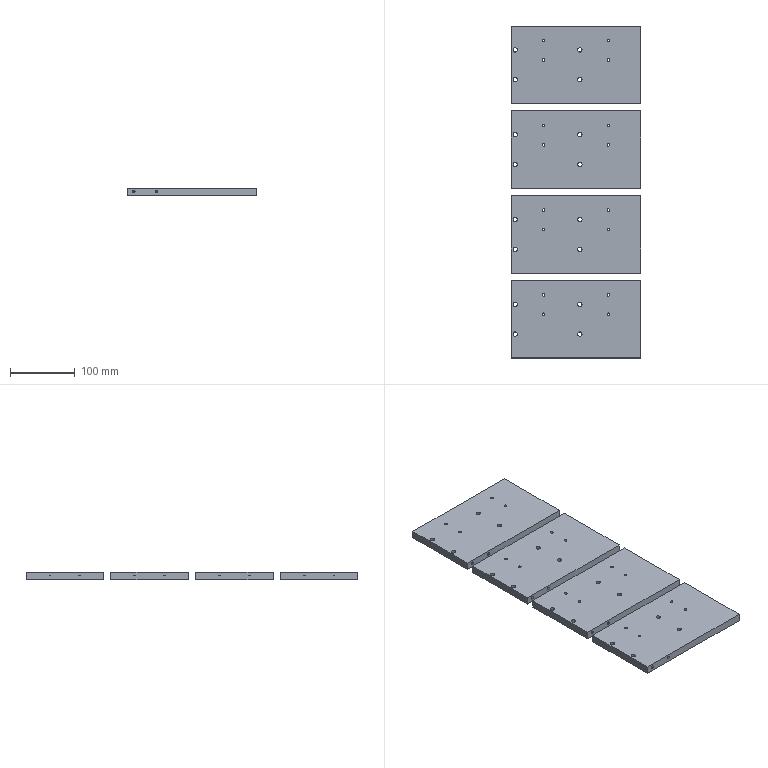CAM job | NX | 3-axis milling, drilling | part box 200 x 513 x 12 mm | stock box 205 x 518 x 12 mm
Tools:
number,name,description,diameter,corner_radius,flute_length,length,flutes
6,D6,平底铣刀-粗,6.0,0.0,25.0,75.0,2
9,D10,平底铣刀-粗,10.0,0.0,35.0,75.0,2
17,D3-J,平底铣刀-精,3.0,0.0,50.0,75.0,2
7,D6-J,平底铣刀-精,6.0,0.0,25.0,75.0,2
2,D6_CHAMFERCUTTER,倒角刀,6.0,0.0,3.0,25.0,2
14,ZT4.2,钻头,4.2,0.0,35.0,50.0,2
18,ZT6.6,钻头,6.6,0.0,35.0,50.0,2
Operations:
program,operation,operation_type,tool,method,geometry_group,spindle_rpm,surface_speed,feed_per_tooth,feed_cut,feed_plunge,cut_length_mm,path_length_mm,cut_time_min,machine_time_min
A,SPOTDRILL,Operation,D6_CHAMFERCUTTER,METHOD,W-A,3000.0,56.549,0.0333,200.0,0.0,80.0,1735.793,0.4,0.5656
A,DRILLHOLE,Operation,ZT4.2,METHOD,W-A,3000.0,38.924,0.0167,100.0,0.0,203.2,1406.568,2.032,2.152
A,DRILLHOLE_2,Operation,ZT6.6,METHOD,W-A,2500.0,51.836,0.03,150.0,0.0,203.2,1439.527,1.355,1.478
A,HOLEROUGH_1,CylinderMilling,D6,METHOD,W-A,6000.0,113.097,0.1667,2000.0,100.0,3789.89,5526.89,1.895,2.069
A,CONTOURROUGH_2,VolumeBased25DMillingOperation,D10,METHOD,W-A,6000.0,188.0,0.25,4000.0,80.0,67210.442,68064.644,16.803,16.888
A,HOLESIDE_1,CylinderMilling,D6-J,METHOD,W-A,6000.0,113.097,0.0667,800.0,100.0,347.068,2197.668,0.4338,0.6189
A,FLOORWALLSPIRALFINISH-MID_COPY,VolumeBased25DMillingOperation,D3-J,SPIRALFINISH-DEPTHK-STEPG,W-A,8000.0,75.398,0.0312,500.0,100.0,2564.107,4317.996,5.128,5.304
A,FLOORWALLSPIRALFINISH-MID_COPY_COPY,VolumeBased25DMillingOperation,D3-J,SPIRALFINISH-DEPTHK-STEPG,W-A,8000.0,75.398,0.0312,500.0,100.0,3454.469,5340.637,6.909,7.098
A,BODYONLY,SurfaceContour,D6_CHAMFERCUTTER,METHOD,W-A,6000.0,113.0,0.125,1200.0,100.0,2629.259,3005.71,2.191,2.229
A,DRILLCHAMFER_1,Operation,D6_CHAMFERCUTTER,METHOD,W-A,5000.0,94.248,0.015,150.0,0.0,90.672,1212.854,0.6045,0.7167
A,MILLCHAMFER_1,PlanarMilling,D6_CHAMFERCUTTER,METHOD,W-A,6000.0,113.097,0.05,600.0,100.0,558.569,2224.715,0.9309,1.098
A,CONTOURSEMI_2,VolumeBased25DMillingOperation,D6-J,METHOD,W-A,6000.0,113.0,0.0833,1000.0,100.0,2655.063,3492.519,2.655,2.739
A,CONTOURFINISH_2,VolumeBased25DMillingOperation,D6-J,METHOD,W-A,6000.0,113.0,0.0833,1000.0,100.0,2654.263,3493.951,2.654,2.738